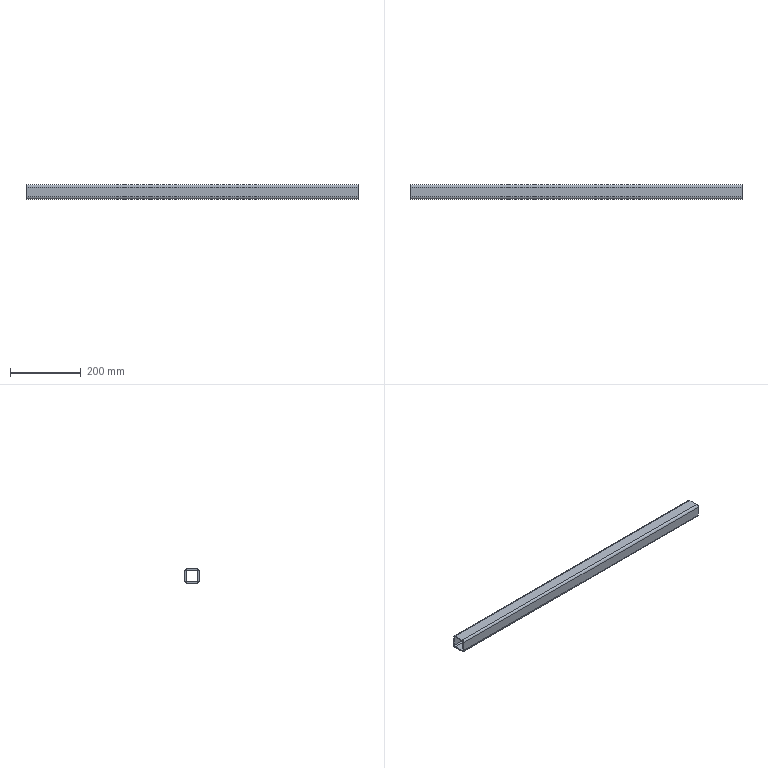Part | SolidWorks | features SavedExtBody 1 | 1 solid | 18 faces | box 940 x 40 x 40 mm | volume 417990 mm3 | plane 10 | cylinder 8 | commonest cylinder face diameters 6.4 x4 12.8 x4
STEP:
#1=CARTESIAN_POINT('',(-1000.,13.6,-450.));
#2=VERTEX_POINT('',#1);
#3=CARTESIAN_POINT('',(-1000.,20.,-443.6));
#4=VERTEX_POINT('',#3);
#5=CARTESIAN_POINT('',(-1000.,13.6,-443.6));
#6=DIRECTION('',(1.,0.,0.));
#7=DIRECTION('',(0.,1.,0.));
#8=AXIS2_PLACEMENT_3D('',#5,#6,#7);
#9=CIRCLE('',#8,6.4);
#10=EDGE_CURVE('',#2,#4,#9,.T.);
#11=ORIENTED_EDGE('',*,*,#10,.F.);
#12=CARTESIAN_POINT('',(-1940.,13.6,-450.));
#13=VERTEX_POINT('',#12);
#14=CARTESIAN_POINT('',(-980.,13.6,-450.));
#15=DIRECTION('',(-1.,0.,0.));
#16=VECTOR('',#15,1000.);
#17=LINE('',#14,#16);
#18=EDGE_CURVE('',#2,#13,#17,.T.);
#19=ORIENTED_EDGE('',*,*,#18,.T.);
#20=CARTESIAN_POINT('',(-1940.,20.,-443.6));
#21=VERTEX_POINT('',#20);
#22=CARTESIAN_POINT('',(-1940.,13.6,-443.6));
#23=DIRECTION('',(-1.,0.,0.));
#24=DIRECTION('',(0.,-1.,0.));
#25=AXIS2_PLACEMENT_3D('',#22,#23,#24);
#26=CIRCLE('',#25,6.4);
#27=EDGE_CURVE('',#21,#13,#26,.T.);
#28=ORIENTED_EDGE('',*,*,#27,.F.);
#29=CARTESIAN_POINT('',(-980.,20.,-443.6));
#30=DIRECTION('',(-1.,0.,0.));
#31=VECTOR('',#30,1000.);
#32=LINE('',#29,#31);
#33=EDGE_CURVE('',#4,#21,#32,.T.);
#34=ORIENTED_EDGE('',*,*,#33,.F.);
#35=EDGE_LOOP('',(#11,#19,#28,#34));
#36=FACE_OUTER_BOUND('',#35,.T.);
#37=CARTESIAN_POINT('',(-980.,13.6,-443.6));
#38=DIRECTION('',(-1.,0.,0.));
#39=DIRECTION('',(0.,0.,1.));
#40=AXIS2_PLACEMENT_3D('',#37,#38,#39);
#41=CYLINDRICAL_SURFACE('',#40,6.4);
#42=ADVANCED_FACE('',(#36),#41,.T.);
#43=CARTESIAN_POINT('',(-1000.,20.,-416.4));
#44=VERTEX_POINT('',#43);
#45=CARTESIAN_POINT('',(-1000.,20.,430.));
#46=DIRECTION('',(0.,0.,-1.));
#47=VECTOR('',#46,1000.);
#48=LINE('',#45,#47);
#49=EDGE_CURVE('',#44,#4,#48,.T.);
#50=ORIENTED_EDGE('',*,*,#49,.T.);
#51=ORIENTED_EDGE('',*,*,#33,.T.);
#52=CARTESIAN_POINT('',(-1940.,20.,-416.4));
#53=VERTEX_POINT('',#52);
#54=CARTESIAN_POINT('',(-1940.,20.,430.));
#55=DIRECTION('',(0.,0.,-1.));
#56=VECTOR('',#55,1000.);
#57=LINE('',#54,#56);
#58=EDGE_CURVE('',#53,#21,#57,.T.);
#59=ORIENTED_EDGE('',*,*,#58,.F.);
#60=CARTESIAN_POINT('',(-980.,20.,-416.4));
#61=DIRECTION('',(-1.,0.,0.));
#62=VECTOR('',#61,1000.);
#63=LINE('',#60,#62);
#64=EDGE_CURVE('',#44,#53,#63,.T.);
#65=ORIENTED_EDGE('',*,*,#64,.F.);
#66=EDGE_LOOP('',(#50,#51,#59,#65));
#67=FACE_OUTER_BOUND('',#66,.T.);
#68=CARTESIAN_POINT('',(-980.,20.,-443.6));
#69=DIRECTION('',(0.,-1.,0.));
#70=DIRECTION('',(0.,0.,-1.));
#71=AXIS2_PLACEMENT_3D('',#68,#69,#70);
#72=PLANE('',#71);
#73=ADVANCED_FACE('',(#67),#72,.F.);
#74=CARTESIAN_POINT('',(-1000.,13.6,-410.));
#75=VERTEX_POINT('',#74);
#76=CARTESIAN_POINT('',(-1000.,13.6,-416.4));
#77=DIRECTION('',(1.,0.,0.));
#78=DIRECTION('',(0.,1.,0.));
#79=AXIS2_PLACEMENT_3D('',#76,#77,#78);
#80=CIRCLE('',#79,6.4);
#81=EDGE_CURVE('',#44,#75,#80,.T.);
#82=ORIENTED_EDGE('',*,*,#81,.F.);
#83=ORIENTED_EDGE('',*,*,#64,.T.);
#84=CARTESIAN_POINT('',(-1940.,13.6,-410.));
#85=VERTEX_POINT('',#84);
#86=CARTESIAN_POINT('',(-1940.,13.6,-416.4));
#87=DIRECTION('',(-1.,0.,0.));
#88=DIRECTION('',(0.,-1.,0.));
#89=AXIS2_PLACEMENT_3D('',#86,#87,#88);
#90=CIRCLE('',#89,6.4);
#91=EDGE_CURVE('',#85,#53,#90,.T.);
#92=ORIENTED_EDGE('',*,*,#91,.F.);
#93=CARTESIAN_POINT('',(-980.,13.6,-410.));
#94=DIRECTION('',(-1.,0.,0.));
#95=VECTOR('',#94,1000.);
#96=LINE('',#93,#95);
#97=EDGE_CURVE('',#75,#85,#96,.T.);
#98=ORIENTED_EDGE('',*,*,#97,.F.);
#99=EDGE_LOOP('',(#82,#83,#92,#98));
#100=FACE_OUTER_BOUND('',#99,.T.);
#101=CARTESIAN_POINT('',(-980.,13.6,-416.4));
#102=DIRECTION('',(-1.,0.,0.));
#103=DIRECTION('',(0.,0.,1.));
#104=AXIS2_PLACEMENT_3D('',#101,#102,#103);
#105=CYLINDRICAL_SURFACE('',#104,6.4);
#106=ADVANCED_FACE('',(#100),#105,.T.);
#107=CARTESIAN_POINT('',(-1000.,-13.6,-410.));
#108=VERTEX_POINT('',#107);
#109=CARTESIAN_POINT('',(-1000.,-13.6,-410.));
#110=DIRECTION('',(0.,-1.,0.));
#111=VECTOR('',#110,1000.);
#112=LINE('',#109,#111);
#113=EDGE_CURVE('',#75,#108,#112,.T.);
#114=ORIENTED_EDGE('',*,*,#113,.F.);
#115=ORIENTED_EDGE('',*,*,#97,.T.);
#116=CARTESIAN_POINT('',(-1940.,-13.6,-410.));
#117=VERTEX_POINT('',#116);
#118=CARTESIAN_POINT('',(-1940.,-13.6,-410.));
#119=DIRECTION('',(0.,1.,0.));
#120=VECTOR('',#119,1000.);
#121=LINE('',#118,#120);
#122=EDGE_CURVE('',#117,#85,#121,.T.);
#123=ORIENTED_EDGE('',*,*,#122,.F.);
#124=CARTESIAN_POINT('',(-980.,-13.6,-410.));
#125=DIRECTION('',(-1.,0.,0.));
#126=VECTOR('',#125,1000.);
#127=LINE('',#124,#126);
#128=EDGE_CURVE('',#108,#117,#127,.T.);
#129=ORIENTED_EDGE('',*,*,#128,.F.);
#130=EDGE_LOOP('',(#114,#115,#123,#129));
#131=FACE_OUTER_BOUND('',#130,.T.);
#132=CARTESIAN_POINT('',(-980.,-13.6,-410.));
#133=DIRECTION('',(0.,0.,-1.));
#134=DIRECTION('',(0.,1.,0.));
#135=AXIS2_PLACEMENT_3D('',#132,#133,#134);
#136=PLANE('',#135);
#137=ADVANCED_FACE('',(#131),#136,.F.);
#138=CARTESIAN_POINT('',(-1000.,-20.,-416.4));
#139=VERTEX_POINT('',#138);
#140=CARTESIAN_POINT('',(-1000.,-13.6,-416.4));
#141=DIRECTION('',(1.,0.,0.));
#142=DIRECTION('',(0.,1.,0.));
#143=AXIS2_PLACEMENT_3D('',#140,#141,#142);
#144=CIRCLE('',#143,6.4);
#145=EDGE_CURVE('',#108,#139,#144,.T.);
#146=ORIENTED_EDGE('',*,*,#145,.F.);
#147=ORIENTED_EDGE('',*,*,#128,.T.);
#148=CARTESIAN_POINT('',(-1940.,-20.,-416.4));
#149=VERTEX_POINT('',#148);
#150=CARTESIAN_POINT('',(-1940.,-13.6,-416.4));
#151=DIRECTION('',(-1.,0.,0.));
#152=DIRECTION('',(0.,-1.,0.));
#153=AXIS2_PLACEMENT_3D('',#150,#151,#152);
#154=CIRCLE('',#153,6.4);
#155=EDGE_CURVE('',#149,#117,#154,.T.);
#156=ORIENTED_EDGE('',*,*,#155,.F.);
#157=CARTESIAN_POINT('',(-980.,-20.,-416.4));
#158=DIRECTION('',(-1.,0.,0.));
#159=VECTOR('',#158,1000.);
#160=LINE('',#157,#159);
#161=EDGE_CURVE('',#139,#149,#160,.T.);
#162=ORIENTED_EDGE('',*,*,#161,.F.);
#163=EDGE_LOOP('',(#146,#147,#156,#162));
#164=FACE_OUTER_BOUND('',#163,.T.);
#165=CARTESIAN_POINT('',(-980.,-13.6,-416.4));
#166=DIRECTION('',(-1.,0.,0.));
#167=DIRECTION('',(0.,0.,1.));
#168=AXIS2_PLACEMENT_3D('',#165,#166,#167);
#169=CYLINDRICAL_SURFACE('',#168,6.4);
#170=ADVANCED_FACE('',(#164),#169,.T.);
#171=CARTESIAN_POINT('',(-1000.,-20.,-443.6));
#172=VERTEX_POINT('',#171);
#173=CARTESIAN_POINT('',(-1000.,-20.,430.));
#174=DIRECTION('',(0.,0.,-1.));
#175=VECTOR('',#174,1000.);
#176=LINE('',#173,#175);
#177=EDGE_CURVE('',#139,#172,#176,.T.);
#178=ORIENTED_EDGE('',*,*,#177,.F.);
#179=ORIENTED_EDGE('',*,*,#161,.T.);
#180=CARTESIAN_POINT('',(-1940.,-20.,-443.6));
#181=VERTEX_POINT('',#180);
#182=CARTESIAN_POINT('',(-1940.,-20.,430.));
#183=DIRECTION('',(0.,0.,-1.));
#184=VECTOR('',#183,1000.);
#185=LINE('',#182,#184);
#186=EDGE_CURVE('',#149,#181,#185,.T.);
#187=ORIENTED_EDGE('',*,*,#186,.T.);
#188=CARTESIAN_POINT('',(-980.,-20.,-443.6));
#189=DIRECTION('',(-1.,0.,0.));
#190=VECTOR('',#189,1000.);
#191=LINE('',#188,#190);
#192=EDGE_CURVE('',#172,#181,#191,.T.);
#193=ORIENTED_EDGE('',*,*,#192,.F.);
#194=EDGE_LOOP('',(#178,#179,#187,#193));
#195=FACE_OUTER_BOUND('',#194,.T.);
#196=CARTESIAN_POINT('',(-980.,-20.,-416.4));
#197=DIRECTION('',(0.,1.,0.));
#198=DIRECTION('',(0.,0.,1.));
#199=AXIS2_PLACEMENT_3D('',#196,#197,#198);
#200=PLANE('',#199);
#201=ADVANCED_FACE('',(#195),#200,.F.);
#202=CARTESIAN_POINT('',(-1000.,-13.6,-450.));
#203=VERTEX_POINT('',#202);
#204=CARTESIAN_POINT('',(-1000.,-13.6,-443.6));
#205=DIRECTION('',(1.,0.,0.));
#206=DIRECTION('',(0.,1.,0.));
#207=AXIS2_PLACEMENT_3D('',#204,#205,#206);
#208=CIRCLE('',#207,6.4);
#209=EDGE_CURVE('',#172,#203,#208,.T.);
#210=ORIENTED_EDGE('',*,*,#209,.F.);
#211=ORIENTED_EDGE('',*,*,#192,.T.);
#212=CARTESIAN_POINT('',(-1940.,-13.6,-450.));
#213=VERTEX_POINT('',#212);
#214=CARTESIAN_POINT('',(-1940.,-13.6,-443.6));
#215=DIRECTION('',(-1.,0.,0.));
#216=DIRECTION('',(0.,-1.,0.));
#217=AXIS2_PLACEMENT_3D('',#214,#215,#216);
#218=CIRCLE('',#217,6.4);
#219=EDGE_CURVE('',#213,#181,#218,.T.);
#220=ORIENTED_EDGE('',*,*,#219,.F.);
#221=CARTESIAN_POINT('',(-980.,-13.6,-450.));
#222=DIRECTION('',(-1.,0.,0.));
#223=VECTOR('',#222,1000.);
#224=LINE('',#221,#223);
#225=EDGE_CURVE('',#203,#213,#224,.T.);
#226=ORIENTED_EDGE('',*,*,#225,.F.);
#227=EDGE_LOOP('',(#210,#211,#220,#226));
#228=FACE_OUTER_BOUND('',#227,.T.);
#229=CARTESIAN_POINT('',(-980.,-13.6,-443.6));
#230=DIRECTION('',(-1.,0.,0.));
#231=DIRECTION('',(0.,0.,1.));
#232=AXIS2_PLACEMENT_3D('',#229,#230,#231);
#233=CYLINDRICAL_SURFACE('',#232,6.4);
#234=ADVANCED_FACE('',(#228),#233,.T.);
#235=CARTESIAN_POINT('',(-1000.,16.8,-416.4));
#236=VERTEX_POINT('',#235);
#237=CARTESIAN_POINT('',(-1940.,16.8,-416.4));
#238=VERTEX_POINT('',#237);
#239=CARTESIAN_POINT('',(-980.,16.8,-416.4));
#240=DIRECTION('',(-1.,0.,0.));
#241=VECTOR('',#240,1000.);
#242=LINE('',#239,#241);
#243=EDGE_CURVE('',#236,#238,#242,.T.);
#244=ORIENTED_EDGE('',*,*,#243,.F.);
#245=CARTESIAN_POINT('',(-1000.,13.6,-413.2));
#246=VERTEX_POINT('',#245);
#247=CARTESIAN_POINT('',(-1000.,13.6,-416.4));
#248=DIRECTION('',(1.,0.,0.));
#249=DIRECTION('',(0.,1.,0.));
#250=AXIS2_PLACEMENT_3D('',#247,#248,#249);
#251=CIRCLE('',#250,3.2);
#252=EDGE_CURVE('',#236,#246,#251,.T.);
#253=ORIENTED_EDGE('',*,*,#252,.T.);
#254=CARTESIAN_POINT('',(-1940.,13.6,-413.2));
#255=VERTEX_POINT('',#254);
#256=CARTESIAN_POINT('',(-980.,13.6,-413.2));
#257=DIRECTION('',(-1.,0.,0.));
#258=VECTOR('',#257,1000.);
#259=LINE('',#256,#258);
#260=EDGE_CURVE('',#246,#255,#259,.T.);
#261=ORIENTED_EDGE('',*,*,#260,.T.);
#262=CARTESIAN_POINT('',(-1940.,13.6,-416.4));
#263=DIRECTION('',(-1.,0.,0.));
#264=DIRECTION('',(0.,-1.,0.));
#265=AXIS2_PLACEMENT_3D('',#262,#263,#264);
#266=CIRCLE('',#265,3.2);
#267=EDGE_CURVE('',#255,#238,#266,.T.);
#268=ORIENTED_EDGE('',*,*,#267,.T.);
#269=EDGE_LOOP('',(#244,#253,#261,#268));
#270=FACE_OUTER_BOUND('',#269,.T.);
#271=CARTESIAN_POINT('',(-980.,13.6,-416.4));
#272=DIRECTION('',(-1.,0.,0.));
#273=DIRECTION('',(0.,0.,1.));
#274=AXIS2_PLACEMENT_3D('',#271,#272,#273);
#275=CYLINDRICAL_SURFACE('',#274,3.2);
#276=ADVANCED_FACE('',(#270),#275,.F.);
#277=CARTESIAN_POINT('',(-1000.,16.8,-443.6));
#278=VERTEX_POINT('',#277);
#279=CARTESIAN_POINT('',(-1940.,16.8,-443.6));
#280=VERTEX_POINT('',#279);
#281=CARTESIAN_POINT('',(-980.,16.8,-443.6));
#282=DIRECTION('',(-1.,0.,0.));
#283=VECTOR('',#282,1000.);
#284=LINE('',#281,#283);
#285=EDGE_CURVE('',#278,#280,#284,.T.);
#286=ORIENTED_EDGE('',*,*,#285,.F.);
#287=CARTESIAN_POINT('',(-1000.,16.8,-443.6));
#288=DIRECTION('',(0.,0.,1.));
#289=VECTOR('',#288,1000.);
#290=LINE('',#287,#289);
#291=EDGE_CURVE('',#278,#236,#290,.T.);
#292=ORIENTED_EDGE('',*,*,#291,.T.);
#293=ORIENTED_EDGE('',*,*,#243,.T.);
#294=CARTESIAN_POINT('',(-1940.,16.8,-443.6));
#295=DIRECTION('',(0.,0.,-1.));
#296=VECTOR('',#295,1000.);
#297=LINE('',#294,#296);
#298=EDGE_CURVE('',#238,#280,#297,.T.);
#299=ORIENTED_EDGE('',*,*,#298,.T.);
#300=EDGE_LOOP('',(#286,#292,#293,#299));
#301=FACE_OUTER_BOUND('',#300,.T.);
#302=CARTESIAN_POINT('',(-980.,16.8,-443.6));
#303=DIRECTION('',(0.,-1.,0.));
#304=DIRECTION('',(0.,0.,-1.));
#305=AXIS2_PLACEMENT_3D('',#302,#303,#304);
#306=PLANE('',#305);
#307=ADVANCED_FACE('',(#301),#306,.T.);
#308=CARTESIAN_POINT('',(-1000.,13.6,-446.8));
#309=VERTEX_POINT('',#308);
#310=CARTESIAN_POINT('',(-1940.,13.6,-446.8));
#311=VERTEX_POINT('',#310);
#312=CARTESIAN_POINT('',(-980.,13.6,-446.8));
#313=DIRECTION('',(-1.,0.,0.));
#314=VECTOR('',#313,1000.);
#315=LINE('',#312,#314);
#316=EDGE_CURVE('',#309,#311,#315,.T.);
#317=ORIENTED_EDGE('',*,*,#316,.F.);
#318=CARTESIAN_POINT('',(-1000.,13.6,-443.6));
#319=DIRECTION('',(1.,0.,0.));
#320=DIRECTION('',(0.,1.,0.));
#321=AXIS2_PLACEMENT_3D('',#318,#319,#320);
#322=CIRCLE('',#321,3.2);
#323=EDGE_CURVE('',#309,#278,#322,.T.);
#324=ORIENTED_EDGE('',*,*,#323,.T.);
#325=ORIENTED_EDGE('',*,*,#285,.T.);
#326=CARTESIAN_POINT('',(-1940.,13.6,-443.6));
#327=DIRECTION('',(-1.,0.,0.));
#328=DIRECTION('',(0.,-1.,0.));
#329=AXIS2_PLACEMENT_3D('',#326,#327,#328);
#330=CIRCLE('',#329,3.2);
#331=EDGE_CURVE('',#280,#311,#330,.T.);
#332=ORIENTED_EDGE('',*,*,#331,.T.);
#333=EDGE_LOOP('',(#317,#324,#325,#332));
#334=FACE_OUTER_BOUND('',#333,.T.);
#335=CARTESIAN_POINT('',(-980.,13.6,-443.6));
#336=DIRECTION('',(-1.,0.,0.));
#337=DIRECTION('',(0.,0.,1.));
#338=AXIS2_PLACEMENT_3D('',#335,#336,#337);
#339=CYLINDRICAL_SURFACE('',#338,3.2);
#340=ADVANCED_FACE('',(#334),#339,.F.);
#341=CARTESIAN_POINT('',(-1000.,-13.6,-446.8));
#342=VERTEX_POINT('',#341);
#343=CARTESIAN_POINT('',(-1940.,-13.6,-446.8));
#344=VERTEX_POINT('',#343);
#345=CARTESIAN_POINT('',(-980.,-13.6,-446.8));
#346=DIRECTION('',(-1.,0.,0.));
#347=VECTOR('',#346,1000.);
#348=LINE('',#345,#347);
#349=EDGE_CURVE('',#342,#344,#348,.T.);
#350=ORIENTED_EDGE('',*,*,#349,.F.);
#351=CARTESIAN_POINT('',(-1000.,13.6,-446.8));
#352=DIRECTION('',(0.,1.,0.));
#353=VECTOR('',#352,1000.);
#354=LINE('',#351,#353);
#355=EDGE_CURVE('',#342,#309,#354,.T.);
#356=ORIENTED_EDGE('',*,*,#355,.T.);
#357=ORIENTED_EDGE('',*,*,#316,.T.);
#358=CARTESIAN_POINT('',(-1940.,13.6,-446.8));
#359=DIRECTION('',(0.,-1.,0.));
#360=VECTOR('',#359,1000.);
#361=LINE('',#358,#360);
#362=EDGE_CURVE('',#311,#344,#361,.T.);
#363=ORIENTED_EDGE('',*,*,#362,.T.);
#364=EDGE_LOOP('',(#350,#356,#357,#363));
#365=FACE_OUTER_BOUND('',#364,.T.);
#366=CARTESIAN_POINT('',(-980.,13.6,-446.8));
#367=DIRECTION('',(0.,0.,1.));
#368=DIRECTION('',(0.,-1.,0.));
#369=AXIS2_PLACEMENT_3D('',#366,#367,#368);
#370=PLANE('',#369);
#371=ADVANCED_FACE('',(#365),#370,.T.);
#372=CARTESIAN_POINT('',(-1000.,-16.8,-443.6));
#373=VERTEX_POINT('',#372);
#374=CARTESIAN_POINT('',(-1940.,-16.8,-443.6));
#375=VERTEX_POINT('',#374);
#376=CARTESIAN_POINT('',(-980.,-16.8,-443.6));
#377=DIRECTION('',(-1.,0.,0.));
#378=VECTOR('',#377,1000.);
#379=LINE('',#376,#378);
#380=EDGE_CURVE('',#373,#375,#379,.T.);
#381=ORIENTED_EDGE('',*,*,#380,.F.);
#382=CARTESIAN_POINT('',(-1000.,-13.6,-443.6));
#383=DIRECTION('',(1.,0.,0.));
#384=DIRECTION('',(0.,1.,0.));
#385=AXIS2_PLACEMENT_3D('',#382,#383,#384);
#386=CIRCLE('',#385,3.2);
#387=EDGE_CURVE('',#373,#342,#386,.T.);
#388=ORIENTED_EDGE('',*,*,#387,.T.);
#389=ORIENTED_EDGE('',*,*,#349,.T.);
#390=CARTESIAN_POINT('',(-1940.,-13.6,-443.6));
#391=DIRECTION('',(-1.,0.,0.));
#392=DIRECTION('',(0.,-1.,0.));
#393=AXIS2_PLACEMENT_3D('',#390,#391,#392);
#394=CIRCLE('',#393,3.2);
#395=EDGE_CURVE('',#344,#375,#394,.T.);
#396=ORIENTED_EDGE('',*,*,#395,.T.);
#397=EDGE_LOOP('',(#381,#388,#389,#396));
#398=FACE_OUTER_BOUND('',#397,.T.);
#399=CARTESIAN_POINT('',(-980.,-13.6,-443.6));
#400=DIRECTION('',(-1.,0.,0.));
#401=DIRECTION('',(0.,0.,1.));
#402=AXIS2_PLACEMENT_3D('',#399,#400,#401);
#403=CYLINDRICAL_SURFACE('',#402,3.2);
#404=ADVANCED_FACE('',(#398),#403,.F.);
#405=CARTESIAN_POINT('',(-1000.,-16.8,-416.4));
#406=VERTEX_POINT('',#405);
#407=CARTESIAN_POINT('',(-1940.,-16.8,-416.4));
#408=VERTEX_POINT('',#407);
#409=CARTESIAN_POINT('',(-980.,-16.8,-416.4));
#410=DIRECTION('',(-1.,0.,0.));
#411=VECTOR('',#410,1000.);
#412=LINE('',#409,#411);
#413=EDGE_CURVE('',#406,#408,#412,.T.);
#414=ORIENTED_EDGE('',*,*,#413,.F.);
#415=CARTESIAN_POINT('',(-1000.,-16.8,-416.4));
#416=DIRECTION('',(0.,0.,-1.));
#417=VECTOR('',#416,1000.);
#418=LINE('',#415,#417);
#419=EDGE_CURVE('',#406,#373,#418,.T.);
#420=ORIENTED_EDGE('',*,*,#419,.T.);
#421=ORIENTED_EDGE('',*,*,#380,.T.);
#422=CARTESIAN_POINT('',(-1940.,-16.8,-416.4));
#423=DIRECTION('',(0.,0.,1.));
#424=VECTOR('',#423,1000.);
#425=LINE('',#422,#424);
#426=EDGE_CURVE('',#375,#408,#425,.T.);
#427=ORIENTED_EDGE('',*,*,#426,.T.);
#428=EDGE_LOOP('',(#414,#420,#421,#427));
#429=FACE_OUTER_BOUND('',#428,.T.);
#430=CARTESIAN_POINT('',(-980.,-16.8,-416.4));
#431=DIRECTION('',(0.,1.,0.));
#432=DIRECTION('',(0.,0.,1.));
#433=AXIS2_PLACEMENT_3D('',#430,#431,#432);
#434=PLANE('',#433);
#435=ADVANCED_FACE('',(#429),#434,.T.);
#436=CARTESIAN_POINT('',(-1000.,-13.6,-413.2));
#437=VERTEX_POINT('',#436);
#438=CARTESIAN_POINT('',(-1940.,-13.6,-413.2));
#439=VERTEX_POINT('',#438);
#440=CARTESIAN_POINT('',(-980.,-13.6,-413.2));
#441=DIRECTION('',(-1.,0.,0.));
#442=VECTOR('',#441,1000.);
#443=LINE('',#440,#442);
#444=EDGE_CURVE('',#437,#439,#443,.T.);
#445=ORIENTED_EDGE('',*,*,#444,.F.);
#446=CARTESIAN_POINT('',(-1000.,-13.6,-416.4));
#447=DIRECTION('',(1.,0.,0.));
#448=DIRECTION('',(0.,1.,0.));
#449=AXIS2_PLACEMENT_3D('',#446,#447,#448);
#450=CIRCLE('',#449,3.2);
#451=EDGE_CURVE('',#437,#406,#450,.T.);
#452=ORIENTED_EDGE('',*,*,#451,.T.);
#453=ORIENTED_EDGE('',*,*,#413,.T.);
#454=CARTESIAN_POINT('',(-1940.,-13.6,-416.4));
#455=DIRECTION('',(-1.,0.,0.));
#456=DIRECTION('',(0.,-1.,0.));
#457=AXIS2_PLACEMENT_3D('',#454,#455,#456);
#458=CIRCLE('',#457,3.2);
#459=EDGE_CURVE('',#408,#439,#458,.T.);
#460=ORIENTED_EDGE('',*,*,#459,.T.);
#461=EDGE_LOOP('',(#445,#452,#453,#460));
#462=FACE_OUTER_BOUND('',#461,.T.);
#463=CARTESIAN_POINT('',(-980.,-13.6,-416.4));
#464=DIRECTION('',(-1.,0.,0.));
#465=DIRECTION('',(0.,0.,1.));
#466=AXIS2_PLACEMENT_3D('',#463,#464,#465);
#467=CYLINDRICAL_SURFACE('',#466,3.2);
#468=ADVANCED_FACE('',(#462),#467,.F.);
#469=ORIENTED_EDGE('',*,*,#260,.F.);
#470=CARTESIAN_POINT('',(-1000.,-13.6,-413.2));
#471=DIRECTION('',(0.,-1.,0.));
#472=VECTOR('',#471,1000.);
#473=LINE('',#470,#472);
#474=EDGE_CURVE('',#246,#437,#473,.T.);
#475=ORIENTED_EDGE('',*,*,#474,.T.);
#476=ORIENTED_EDGE('',*,*,#444,.T.);
#477=CARTESIAN_POINT('',(-1940.,-13.6,-413.2));
#478=DIRECTION('',(0.,1.,0.));
#479=VECTOR('',#478,1000.);
#480=LINE('',#477,#479);
#481=EDGE_CURVE('',#439,#255,#480,.T.);
#482=ORIENTED_EDGE('',*,*,#481,.T.);
#483=EDGE_LOOP('',(#469,#475,#476,#482));
#484=FACE_OUTER_BOUND('',#483,.T.);
#485=CARTESIAN_POINT('',(-980.,-13.6,-413.2));
#486=DIRECTION('',(0.,0.,-1.));
#487=DIRECTION('',(0.,1.,0.));
#488=AXIS2_PLACEMENT_3D('',#485,#486,#487);
#489=PLANE('',#488);
#490=ADVANCED_FACE('',(#484),#489,.T.);
#491=CARTESIAN_POINT('',(-1000.,13.6,-450.));
#492=DIRECTION('',(0.,1.,0.));
#493=VECTOR('',#492,1000.);
#494=LINE('',#491,#493);
#495=EDGE_CURVE('',#203,#2,#494,.T.);
#496=ORIENTED_EDGE('',*,*,#495,.F.);
#497=ORIENTED_EDGE('',*,*,#225,.T.);
#498=CARTESIAN_POINT('',(-1940.,13.6,-450.));
#499=DIRECTION('',(0.,-1.,0.));
#500=VECTOR('',#499,1000.);
#501=LINE('',#498,#500);
#502=EDGE_CURVE('',#13,#213,#501,.T.);
#503=ORIENTED_EDGE('',*,*,#502,.F.);
#504=ORIENTED_EDGE('',*,*,#18,.F.);
#505=EDGE_LOOP('',(#496,#497,#503,#504));
#506=FACE_OUTER_BOUND('',#505,.T.);
#507=CARTESIAN_POINT('',(-980.,13.6,-450.));
#508=DIRECTION('',(0.,0.,1.));
#509=DIRECTION('',(0.,-1.,0.));
#510=AXIS2_PLACEMENT_3D('',#507,#508,#509);
#511=PLANE('',#510);
#512=ADVANCED_FACE('',(#506),#511,.F.);
#513=ORIENTED_EDGE('',*,*,#481,.F.);
#514=ORIENTED_EDGE('',*,*,#459,.F.);
#515=ORIENTED_EDGE('',*,*,#426,.F.);
#516=ORIENTED_EDGE('',*,*,#395,.F.);
#517=ORIENTED_EDGE('',*,*,#362,.F.);
#518=ORIENTED_EDGE('',*,*,#331,.F.);
#519=ORIENTED_EDGE('',*,*,#298,.F.);
#520=ORIENTED_EDGE('',*,*,#267,.F.);
#521=EDGE_LOOP('',(#513,#514,#515,#516,#517,#518,#519,#520));
#522=FACE_BOUND('',#521,.T.);
#523=ORIENTED_EDGE('',*,*,#91,.T.);
#524=ORIENTED_EDGE('',*,*,#58,.T.);
#525=ORIENTED_EDGE('',*,*,#27,.T.);
#526=ORIENTED_EDGE('',*,*,#502,.T.);
#527=ORIENTED_EDGE('',*,*,#219,.T.);
#528=ORIENTED_EDGE('',*,*,#186,.F.);
#529=ORIENTED_EDGE('',*,*,#155,.T.);
#530=ORIENTED_EDGE('',*,*,#122,.T.);
#531=EDGE_LOOP('',(#523,#524,#525,#526,#527,#528,#529,#530));
#532=FACE_OUTER_BOUND('',#531,.T.);
#533=CARTESIAN_POINT('',(-1940.,13.6,430.));
#534=DIRECTION('',(-1.,0.,0.));
#535=DIRECTION('',(0.,-1.,0.));
#536=AXIS2_PLACEMENT_3D('',#533,#534,#535);
#537=PLANE('',#536);
#538=ADVANCED_FACE('',(#522,#532),#537,.T.);
#539=ORIENTED_EDGE('',*,*,#291,.F.);
#540=ORIENTED_EDGE('',*,*,#323,.F.);
#541=ORIENTED_EDGE('',*,*,#355,.F.);
#542=ORIENTED_EDGE('',*,*,#387,.F.);
#543=ORIENTED_EDGE('',*,*,#419,.F.);
#544=ORIENTED_EDGE('',*,*,#451,.F.);
#545=ORIENTED_EDGE('',*,*,#474,.F.);
#546=ORIENTED_EDGE('',*,*,#252,.F.);
#547=EDGE_LOOP('',(#539,#540,#541,#542,#543,#544,#545,#546));
#548=FACE_BOUND('',#547,.T.);
#549=ORIENTED_EDGE('',*,*,#81,.T.);
#550=ORIENTED_EDGE('',*,*,#113,.T.);
#551=ORIENTED_EDGE('',*,*,#145,.T.);
#552=ORIENTED_EDGE('',*,*,#177,.T.);
#553=ORIENTED_EDGE('',*,*,#209,.T.);
#554=ORIENTED_EDGE('',*,*,#495,.T.);
#555=ORIENTED_EDGE('',*,*,#10,.T.);
#556=ORIENTED_EDGE('',*,*,#49,.F.);
#557=EDGE_LOOP('',(#549,#550,#551,#552,#553,#554,#555,#556));
#558=FACE_OUTER_BOUND('',#557,.T.);
#559=CARTESIAN_POINT('',(-1000.,-13.6,430.));
#560=DIRECTION('',(1.,0.,0.));
#561=DIRECTION('',(0.,1.,0.));
#562=AXIS2_PLACEMENT_3D('',#559,#560,#561);
#563=PLANE('',#562);
#564=ADVANCED_FACE('',(#548,#558),#563,.T.);
#565=CLOSED_SHELL('',(#42,#73,#106,#137,#170,#201,#234,#276,#307,#340,#371,#404,#435,#468,#490,#512,#538,#564));
#566=MANIFOLD_SOLID_BREP('',#565);
#567=CARTESIAN_POINT('',(0.,0.,0.));
#568=DIRECTION('',(0.,0.,1.));
#569=DIRECTION('',(1.,0.,0.));
#570=AXIS2_PLACEMENT_3D('',#567,#568,#569);
#571=(LENGTH_UNIT()NAMED_UNIT(*)SI_UNIT(.MILLI.,.METRE.));
#572=UNCERTAINTY_MEASURE_WITH_UNIT(LENGTH_MEASURE(0.00001),#571,'','');
#573=(NAMED_UNIT(*)PLANE_ANGLE_UNIT()SI_UNIT($,.RADIAN.));
#574=(NAMED_UNIT(*)SI_UNIT($,.STERADIAN.)SOLID_ANGLE_UNIT());
#575=(GEOMETRIC_REPRESENTATION_CONTEXT(3)GLOBAL_UNCERTAINTY_ASSIGNED_CONTEXT((#572))GLOBAL_UNIT_ASSIGNED_CONTEXT((#571,#573,#574))REPRESENTATION_CONTEXT('',''));
#576=ADVANCED_BREP_SHAPE_REPRESENTATION('',(#566,#570),#575);